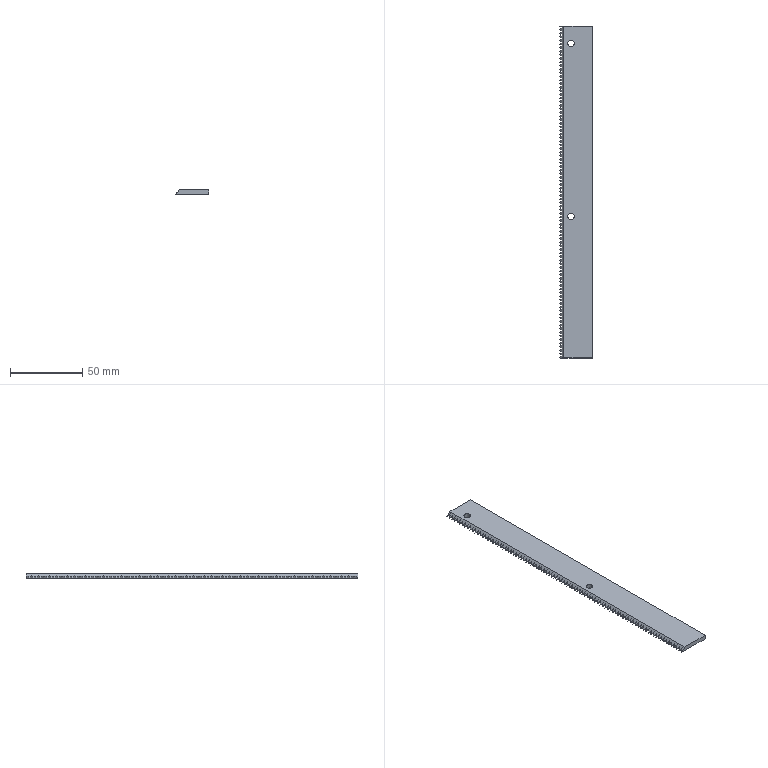Part | SolidWorks | features Cut 2, Chamfer 1, Extrusion 1, ICE 1, LPattern 1 | 1 solid | 195 faces | box 23 x 230.294 x 3 mm | volume 14437 mm3 | plane 191 | cylinder 4 | commonest cylinder face diameters 4.6 x4